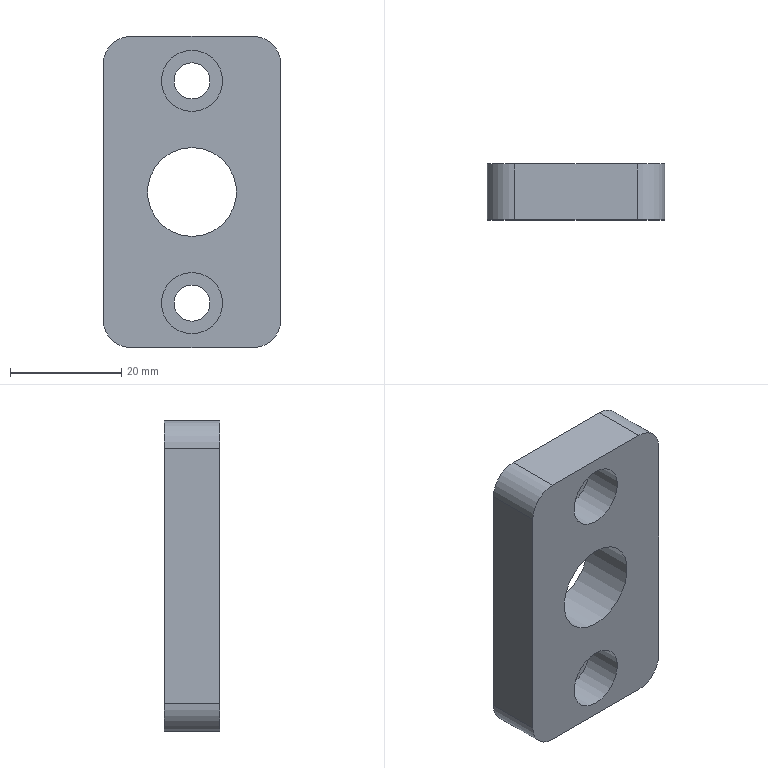Part | STEP file | B-PLATE-INSERT_id78_x_t | 1 solid | 17 faces | box 32 x 10 x 56 mm | volume 14165 mm3 | cylinder 9 | plane 8 | commonest cylinder face diameters 10 x4 6.5 x2 11 x2 16 x1
STEP:
#1=CARTESIAN_POINT('',(-115.,-113.5,-20.5));
#2=VERTEX_POINT('',#1);
#3=CARTESIAN_POINT('',(-115.,-113.5,-15.));
#4=DIRECTION('',(0.,-1.,0.));
#5=DIRECTION('',(0.,0.,-1.));
#6=AXIS2_PLACEMENT_3D('',#3,#4,#5);
#7=CIRCLE('',#6,5.5);
#8=EDGE_CURVE('',#2,#2,#7,.T.);
#9=ORIENTED_EDGE('',*,*,#8,.F.);
#10=EDGE_LOOP('',(#9));
#11=FACE_BOUND('',#10,.T.);
#12=CARTESIAN_POINT('',(-115.,-120.5,-20.5));
#13=VERTEX_POINT('',#12);
#14=CARTESIAN_POINT('',(-115.,-120.5,-15.));
#15=DIRECTION('',(0.,1.,0.));
#16=DIRECTION('',(0.,0.,-1.));
#17=AXIS2_PLACEMENT_3D('',#14,#15,#16);
#18=CIRCLE('',#17,5.5);
#19=EDGE_CURVE('',#13,#13,#18,.T.);
#20=ORIENTED_EDGE('',*,*,#19,.F.);
#21=EDGE_LOOP('',(#20));
#22=FACE_BOUND('',#21,.T.);
#23=CARTESIAN_POINT('',(-115.,-120.5,-15.));
#24=DIRECTION('',(0.,-1.,0.));
#25=DIRECTION('',(0.,0.,-1.));
#26=AXIS2_PLACEMENT_3D('',#23,#24,#25);
#27=CYLINDRICAL_SURFACE('',#26,5.5);
#28=ADVANCED_FACE('',(#11,#22),#27,.F.);
#29=CARTESIAN_POINT('',(-115.,-113.5,-60.5));
#30=VERTEX_POINT('',#29);
#31=CARTESIAN_POINT('',(-115.,-113.5,-55.));
#32=DIRECTION('',(0.,-1.,0.));
#33=DIRECTION('',(0.,0.,-1.));
#34=AXIS2_PLACEMENT_3D('',#31,#32,#33);
#35=CIRCLE('',#34,5.5);
#36=EDGE_CURVE('',#30,#30,#35,.T.);
#37=ORIENTED_EDGE('',*,*,#36,.F.);
#38=EDGE_LOOP('',(#37));
#39=FACE_BOUND('',#38,.T.);
#40=CARTESIAN_POINT('',(-115.,-120.5,-60.5));
#41=VERTEX_POINT('',#40);
#42=CARTESIAN_POINT('',(-115.,-120.5,-55.));
#43=DIRECTION('',(0.,1.,0.));
#44=DIRECTION('',(0.,0.,-1.));
#45=AXIS2_PLACEMENT_3D('',#42,#43,#44);
#46=CIRCLE('',#45,5.5);
#47=EDGE_CURVE('',#41,#41,#46,.T.);
#48=ORIENTED_EDGE('',*,*,#47,.F.);
#49=EDGE_LOOP('',(#48));
#50=FACE_BOUND('',#49,.T.);
#51=CARTESIAN_POINT('',(-115.,-120.5,-55.));
#52=DIRECTION('',(0.,-1.,0.));
#53=DIRECTION('',(0.,0.,-1.));
#54=AXIS2_PLACEMENT_3D('',#51,#52,#53);
#55=CYLINDRICAL_SURFACE('',#54,5.5);
#56=ADVANCED_FACE('',(#39,#50),#55,.F.);
#57=CARTESIAN_POINT('',(-115.,-120.5,-43.));
#58=VERTEX_POINT('',#57);
#59=CARTESIAN_POINT('',(-115.,-120.5,-35.));
#60=DIRECTION('',(0.,-1.,0.));
#61=DIRECTION('',(0.,0.,-1.));
#62=AXIS2_PLACEMENT_3D('',#59,#60,#61);
#63=CIRCLE('',#62,8.);
#64=EDGE_CURVE('',#58,#58,#63,.T.);
#65=ORIENTED_EDGE('',*,*,#64,.F.);
#66=EDGE_LOOP('',(#65));
#67=FACE_BOUND('',#66,.T.);
#68=ORIENTED_EDGE('',*,*,#19,.T.);
#69=EDGE_LOOP('',(#68));
#70=FACE_BOUND('',#69,.T.);
#71=ORIENTED_EDGE('',*,*,#47,.T.);
#72=EDGE_LOOP('',(#71));
#73=FACE_BOUND('',#72,.T.);
#74=CARTESIAN_POINT('',(-131.,-120.5,-58.));
#75=VERTEX_POINT('',#74);
#76=CARTESIAN_POINT('',(-131.,-120.5,-12.));
#77=VERTEX_POINT('',#76);
#78=CARTESIAN_POINT('',(-131.,-120.5,-12.));
#79=DIRECTION('',(0.,0.,1.));
#80=VECTOR('',#79,1.);
#81=LINE('',#78,#80);
#82=EDGE_CURVE('',#75,#77,#81,.T.);
#83=ORIENTED_EDGE('',*,*,#82,.F.);
#84=CARTESIAN_POINT('',(-126.,-120.5,-63.));
#85=VERTEX_POINT('',#84);
#86=CARTESIAN_POINT('',(-126.,-120.5,-58.));
#87=DIRECTION('',(0.,1.,0.));
#88=DIRECTION('',(0.,0.,-1.));
#89=AXIS2_PLACEMENT_3D('',#86,#87,#88);
#90=CIRCLE('',#89,5.);
#91=EDGE_CURVE('',#85,#75,#90,.T.);
#92=ORIENTED_EDGE('',*,*,#91,.F.);
#93=CARTESIAN_POINT('',(-104.,-120.5,-63.));
#94=VERTEX_POINT('',#93);
#95=CARTESIAN_POINT('',(-126.,-120.5,-63.));
#96=DIRECTION('',(-1.,0.,0.));
#97=VECTOR('',#96,1.);
#98=LINE('',#95,#97);
#99=EDGE_CURVE('',#94,#85,#98,.T.);
#100=ORIENTED_EDGE('',*,*,#99,.F.);
#101=CARTESIAN_POINT('',(-99.,-120.5,-58.));
#102=VERTEX_POINT('',#101);
#103=CARTESIAN_POINT('',(-104.,-120.5,-58.));
#104=DIRECTION('',(0.,1.,0.));
#105=DIRECTION('',(0.,0.,-1.));
#106=AXIS2_PLACEMENT_3D('',#103,#104,#105);
#107=CIRCLE('',#106,5.);
#108=EDGE_CURVE('',#102,#94,#107,.T.);
#109=ORIENTED_EDGE('',*,*,#108,.F.);
#110=CARTESIAN_POINT('',(-99.,-120.5,-12.));
#111=VERTEX_POINT('',#110);
#112=CARTESIAN_POINT('',(-99.,-120.5,-58.));
#113=DIRECTION('',(0.,0.,-1.));
#114=VECTOR('',#113,1.);
#115=LINE('',#112,#114);
#116=EDGE_CURVE('',#111,#102,#115,.T.);
#117=ORIENTED_EDGE('',*,*,#116,.F.);
#118=CARTESIAN_POINT('',(-104.,-120.5,-7.));
#119=VERTEX_POINT('',#118);
#120=CARTESIAN_POINT('',(-104.,-120.5,-12.));
#121=DIRECTION('',(0.,1.,0.));
#122=DIRECTION('',(0.,0.,-1.));
#123=AXIS2_PLACEMENT_3D('',#120,#121,#122);
#124=CIRCLE('',#123,5.);
#125=EDGE_CURVE('',#119,#111,#124,.T.);
#126=ORIENTED_EDGE('',*,*,#125,.F.);
#127=CARTESIAN_POINT('',(-126.,-120.5,-7.));
#128=VERTEX_POINT('',#127);
#129=CARTESIAN_POINT('',(-104.,-120.5,-7.));
#130=DIRECTION('',(1.,0.,0.));
#131=VECTOR('',#130,1.);
#132=LINE('',#129,#131);
#133=EDGE_CURVE('',#128,#119,#132,.T.);
#134=ORIENTED_EDGE('',*,*,#133,.F.);
#135=CARTESIAN_POINT('',(-126.,-120.5,-12.));
#136=DIRECTION('',(0.,1.,0.));
#137=DIRECTION('',(0.,0.,-1.));
#138=AXIS2_PLACEMENT_3D('',#135,#136,#137);
#139=CIRCLE('',#138,5.);
#140=EDGE_CURVE('',#77,#128,#139,.T.);
#141=ORIENTED_EDGE('',*,*,#140,.F.);
#142=EDGE_LOOP('',(#83,#92,#100,#109,#117,#126,#134,#141));
#143=FACE_BOUND('',#142,.T.);
#144=CARTESIAN_POINT('',(-80.,-120.5,-43.));
#145=DIRECTION('',(0.,-1.,0.));
#146=DIRECTION('',(0.,0.,-1.));
#147=AXIS2_PLACEMENT_3D('',#144,#145,#146);
#148=PLANE('',#147);
#149=ADVANCED_FACE('',(#67,#70,#73,#143),#148,.T.);
#150=CARTESIAN_POINT('',(-115.,-113.5,-18.25));
#151=VERTEX_POINT('',#150);
#152=CARTESIAN_POINT('',(-115.,-113.5,-15.));
#153=DIRECTION('',(0.,1.,0.));
#154=DIRECTION('',(0.,0.,-1.));
#155=AXIS2_PLACEMENT_3D('',#152,#153,#154);
#156=CIRCLE('',#155,3.25);
#157=EDGE_CURVE('',#151,#151,#156,.T.);
#158=ORIENTED_EDGE('',*,*,#157,.T.);
#159=EDGE_LOOP('',(#158));
#160=FACE_BOUND('',#159,.T.);
#161=ORIENTED_EDGE('',*,*,#8,.T.);
#162=EDGE_LOOP('',(#161));
#163=FACE_BOUND('',#162,.T.);
#164=CARTESIAN_POINT('',(-200.,-113.5,-275.));
#165=DIRECTION('',(0.,-1.,0.));
#166=DIRECTION('',(0.,0.,-1.));
#167=AXIS2_PLACEMENT_3D('',#164,#165,#166);
#168=PLANE('',#167);
#169=ADVANCED_FACE('',(#160,#163),#168,.T.);
#170=CARTESIAN_POINT('',(-115.,-113.5,-58.25));
#171=VERTEX_POINT('',#170);
#172=CARTESIAN_POINT('',(-115.,-113.5,-55.));
#173=DIRECTION('',(0.,1.,0.));
#174=DIRECTION('',(0.,0.,-1.));
#175=AXIS2_PLACEMENT_3D('',#172,#173,#174);
#176=CIRCLE('',#175,3.25);
#177=EDGE_CURVE('',#171,#171,#176,.T.);
#178=ORIENTED_EDGE('',*,*,#177,.T.);
#179=EDGE_LOOP('',(#178));
#180=FACE_BOUND('',#179,.T.);
#181=ORIENTED_EDGE('',*,*,#36,.T.);
#182=EDGE_LOOP('',(#181));
#183=FACE_BOUND('',#182,.T.);
#184=CARTESIAN_POINT('',(-200.,-113.5,-275.));
#185=DIRECTION('',(0.,-1.,0.));
#186=DIRECTION('',(0.,0.,-1.));
#187=AXIS2_PLACEMENT_3D('',#184,#185,#186);
#188=PLANE('',#187);
#189=ADVANCED_FACE('',(#180,#183),#188,.T.);
#190=CARTESIAN_POINT('',(-131.,-110.5,-58.));
#191=VERTEX_POINT('',#190);
#192=CARTESIAN_POINT('',(-131.,-110.5,-58.));
#193=DIRECTION('',(0.,-1.,0.));
#194=VECTOR('',#193,1.);
#195=LINE('',#192,#194);
#196=EDGE_CURVE('',#191,#75,#195,.T.);
#197=ORIENTED_EDGE('',*,*,#196,.F.);
#198=CARTESIAN_POINT('',(-126.,-110.5,-63.));
#199=VERTEX_POINT('',#198);
#200=CARTESIAN_POINT('',(-126.,-110.5,-58.));
#201=DIRECTION('',(0.,-1.,0.));
#202=DIRECTION('',(0.,0.,-1.));
#203=AXIS2_PLACEMENT_3D('',#200,#201,#202);
#204=CIRCLE('',#203,5.);
#205=EDGE_CURVE('',#191,#199,#204,.T.);
#206=ORIENTED_EDGE('',*,*,#205,.T.);
#207=CARTESIAN_POINT('',(-126.,-110.5,-63.));
#208=DIRECTION('',(0.,1.,0.));
#209=VECTOR('',#208,1.);
#210=LINE('',#207,#209);
#211=EDGE_CURVE('',#85,#199,#210,.T.);
#212=ORIENTED_EDGE('',*,*,#211,.F.);
#213=ORIENTED_EDGE('',*,*,#91,.T.);
#214=EDGE_LOOP('',(#197,#206,#212,#213));
#215=FACE_OUTER_BOUND('',#214,.T.);
#216=CARTESIAN_POINT('',(-126.,-110.5,-58.));
#217=DIRECTION('',(0.,-1.,0.));
#218=DIRECTION('',(0.,0.,-1.));
#219=AXIS2_PLACEMENT_3D('',#216,#217,#218);
#220=CYLINDRICAL_SURFACE('',#219,5.);
#221=ADVANCED_FACE('',(#215),#220,.T.);
#222=ORIENTED_EDGE('',*,*,#211,.T.);
#223=CARTESIAN_POINT('',(-104.,-110.5,-63.));
#224=VERTEX_POINT('',#223);
#225=CARTESIAN_POINT('',(-200.,-110.5,-63.));
#226=DIRECTION('',(1.,0.,0.));
#227=VECTOR('',#226,1.);
#228=LINE('',#225,#227);
#229=EDGE_CURVE('',#199,#224,#228,.T.);
#230=ORIENTED_EDGE('',*,*,#229,.T.);
#231=CARTESIAN_POINT('',(-104.,-110.5,-63.));
#232=DIRECTION('',(0.,1.,0.));
#233=VECTOR('',#232,1.);
#234=LINE('',#231,#233);
#235=EDGE_CURVE('',#94,#224,#234,.T.);
#236=ORIENTED_EDGE('',*,*,#235,.F.);
#237=ORIENTED_EDGE('',*,*,#99,.T.);
#238=EDGE_LOOP('',(#222,#230,#236,#237));
#239=FACE_OUTER_BOUND('',#238,.T.);
#240=CARTESIAN_POINT('',(-126.,-110.5,-63.));
#241=DIRECTION('',(0.,0.,-1.));
#242=DIRECTION('',(-1.,0.,0.));
#243=AXIS2_PLACEMENT_3D('',#240,#241,#242);
#244=PLANE('',#243);
#245=ADVANCED_FACE('',(#239),#244,.T.);
#246=ORIENTED_EDGE('',*,*,#235,.T.);
#247=CARTESIAN_POINT('',(-99.,-110.5,-58.));
#248=VERTEX_POINT('',#247);
#249=CARTESIAN_POINT('',(-104.,-110.5,-58.));
#250=DIRECTION('',(0.,-1.,0.));
#251=DIRECTION('',(0.,0.,-1.));
#252=AXIS2_PLACEMENT_3D('',#249,#250,#251);
#253=CIRCLE('',#252,5.);
#254=EDGE_CURVE('',#224,#248,#253,.T.);
#255=ORIENTED_EDGE('',*,*,#254,.T.);
#256=CARTESIAN_POINT('',(-99.,-110.5,-58.));
#257=DIRECTION('',(0.,1.,0.));
#258=VECTOR('',#257,1.);
#259=LINE('',#256,#258);
#260=EDGE_CURVE('',#102,#248,#259,.T.);
#261=ORIENTED_EDGE('',*,*,#260,.F.);
#262=ORIENTED_EDGE('',*,*,#108,.T.);
#263=EDGE_LOOP('',(#246,#255,#261,#262));
#264=FACE_OUTER_BOUND('',#263,.T.);
#265=CARTESIAN_POINT('',(-104.,-110.5,-58.));
#266=DIRECTION('',(0.,-1.,0.));
#267=DIRECTION('',(0.,0.,-1.));
#268=AXIS2_PLACEMENT_3D('',#265,#266,#267);
#269=CYLINDRICAL_SURFACE('',#268,5.);
#270=ADVANCED_FACE('',(#264),#269,.T.);
#271=ORIENTED_EDGE('',*,*,#260,.T.);
#272=CARTESIAN_POINT('',(-99.,-110.5,-12.));
#273=VERTEX_POINT('',#272);
#274=CARTESIAN_POINT('',(-99.,-110.5,-275.));
#275=DIRECTION('',(0.,0.,1.));
#276=VECTOR('',#275,1.);
#277=LINE('',#274,#276);
#278=EDGE_CURVE('',#248,#273,#277,.T.);
#279=ORIENTED_EDGE('',*,*,#278,.T.);
#280=CARTESIAN_POINT('',(-99.,-110.5,-12.));
#281=DIRECTION('',(0.,1.,0.));
#282=VECTOR('',#281,1.);
#283=LINE('',#280,#282);
#284=EDGE_CURVE('',#111,#273,#283,.T.);
#285=ORIENTED_EDGE('',*,*,#284,.F.);
#286=ORIENTED_EDGE('',*,*,#116,.T.);
#287=EDGE_LOOP('',(#271,#279,#285,#286));
#288=FACE_OUTER_BOUND('',#287,.T.);
#289=CARTESIAN_POINT('',(-99.,-110.5,-58.));
#290=DIRECTION('',(1.,0.,0.));
#291=DIRECTION('',(0.,0.,-1.));
#292=AXIS2_PLACEMENT_3D('',#289,#290,#291);
#293=PLANE('',#292);
#294=ADVANCED_FACE('',(#288),#293,.T.);
#295=ORIENTED_EDGE('',*,*,#284,.T.);
#296=CARTESIAN_POINT('',(-104.,-110.5,-7.));
#297=VERTEX_POINT('',#296);
#298=CARTESIAN_POINT('',(-104.,-110.5,-12.));
#299=DIRECTION('',(0.,-1.,0.));
#300=DIRECTION('',(0.,0.,-1.));
#301=AXIS2_PLACEMENT_3D('',#298,#299,#300);
#302=CIRCLE('',#301,5.);
#303=EDGE_CURVE('',#273,#297,#302,.T.);
#304=ORIENTED_EDGE('',*,*,#303,.T.);
#305=CARTESIAN_POINT('',(-104.,-110.5,-7.));
#306=DIRECTION('',(0.,1.,0.));
#307=VECTOR('',#306,1.);
#308=LINE('',#305,#307);
#309=EDGE_CURVE('',#119,#297,#308,.T.);
#310=ORIENTED_EDGE('',*,*,#309,.F.);
#311=ORIENTED_EDGE('',*,*,#125,.T.);
#312=EDGE_LOOP('',(#295,#304,#310,#311));
#313=FACE_OUTER_BOUND('',#312,.T.);
#314=CARTESIAN_POINT('',(-104.,-110.5,-12.));
#315=DIRECTION('',(0.,-1.,0.));
#316=DIRECTION('',(0.,0.,-1.));
#317=AXIS2_PLACEMENT_3D('',#314,#315,#316);
#318=CYLINDRICAL_SURFACE('',#317,5.);
#319=ADVANCED_FACE('',(#313),#318,.T.);
#320=ORIENTED_EDGE('',*,*,#309,.T.);
#321=CARTESIAN_POINT('',(-126.,-110.5,-7.));
#322=VERTEX_POINT('',#321);
#323=CARTESIAN_POINT('',(-200.,-110.5,-7.));
#324=DIRECTION('',(-1.,0.,0.));
#325=VECTOR('',#324,1.);
#326=LINE('',#323,#325);
#327=EDGE_CURVE('',#297,#322,#326,.T.);
#328=ORIENTED_EDGE('',*,*,#327,.T.);
#329=CARTESIAN_POINT('',(-126.,-110.5,-7.));
#330=DIRECTION('',(0.,1.,0.));
#331=VECTOR('',#330,1.);
#332=LINE('',#329,#331);
#333=EDGE_CURVE('',#128,#322,#332,.T.);
#334=ORIENTED_EDGE('',*,*,#333,.F.);
#335=ORIENTED_EDGE('',*,*,#133,.T.);
#336=EDGE_LOOP('',(#320,#328,#334,#335));
#337=FACE_OUTER_BOUND('',#336,.T.);
#338=CARTESIAN_POINT('',(-104.,-110.5,-7.));
#339=DIRECTION('',(0.,0.,1.));
#340=DIRECTION('',(1.,0.,0.));
#341=AXIS2_PLACEMENT_3D('',#338,#339,#340);
#342=PLANE('',#341);
#343=ADVANCED_FACE('',(#337),#342,.T.);
#344=ORIENTED_EDGE('',*,*,#333,.T.);
#345=CARTESIAN_POINT('',(-131.,-110.5,-12.));
#346=VERTEX_POINT('',#345);
#347=CARTESIAN_POINT('',(-126.,-110.5,-12.));
#348=DIRECTION('',(0.,-1.,0.));
#349=DIRECTION('',(0.,0.,-1.));
#350=AXIS2_PLACEMENT_3D('',#347,#348,#349);
#351=CIRCLE('',#350,5.);
#352=EDGE_CURVE('',#322,#346,#351,.T.);
#353=ORIENTED_EDGE('',*,*,#352,.T.);
#354=CARTESIAN_POINT('',(-131.,-110.5,-12.));
#355=DIRECTION('',(0.,1.,0.));
#356=VECTOR('',#355,1.);
#357=LINE('',#354,#356);
#358=EDGE_CURVE('',#77,#346,#357,.T.);
#359=ORIENTED_EDGE('',*,*,#358,.F.);
#360=ORIENTED_EDGE('',*,*,#140,.T.);
#361=EDGE_LOOP('',(#344,#353,#359,#360));
#362=FACE_OUTER_BOUND('',#361,.T.);
#363=CARTESIAN_POINT('',(-126.,-110.5,-12.));
#364=DIRECTION('',(0.,-1.,0.));
#365=DIRECTION('',(0.,0.,-1.));
#366=AXIS2_PLACEMENT_3D('',#363,#364,#365);
#367=CYLINDRICAL_SURFACE('',#366,5.);
#368=ADVANCED_FACE('',(#362),#367,.T.);
#369=ORIENTED_EDGE('',*,*,#358,.T.);
#370=CARTESIAN_POINT('',(-131.,-110.5,-275.));
#371=DIRECTION('',(0.,0.,-1.));
#372=VECTOR('',#371,1.);
#373=LINE('',#370,#372);
#374=EDGE_CURVE('',#346,#191,#373,.T.);
#375=ORIENTED_EDGE('',*,*,#374,.T.);
#376=ORIENTED_EDGE('',*,*,#196,.T.);
#377=ORIENTED_EDGE('',*,*,#82,.T.);
#378=EDGE_LOOP('',(#369,#375,#376,#377));
#379=FACE_OUTER_BOUND('',#378,.T.);
#380=CARTESIAN_POINT('',(-131.,-110.5,-12.));
#381=DIRECTION('',(-1.,0.,0.));
#382=DIRECTION('',(0.,0.,1.));
#383=AXIS2_PLACEMENT_3D('',#380,#381,#382);
#384=PLANE('',#383);
#385=ADVANCED_FACE('',(#379),#384,.T.);
#386=CARTESIAN_POINT('',(-115.,-110.5,-18.25));
#387=VERTEX_POINT('',#386);
#388=CARTESIAN_POINT('',(-115.,-110.5,-15.));
#389=DIRECTION('',(0.,1.,0.));
#390=DIRECTION('',(0.,0.,-1.));
#391=AXIS2_PLACEMENT_3D('',#388,#389,#390);
#392=CIRCLE('',#391,3.25);
#393=EDGE_CURVE('',#387,#387,#392,.T.);
#394=ORIENTED_EDGE('',*,*,#393,.T.);
#395=EDGE_LOOP('',(#394));
#396=FACE_BOUND('',#395,.T.);
#397=ORIENTED_EDGE('',*,*,#157,.F.);
#398=EDGE_LOOP('',(#397));
#399=FACE_BOUND('',#398,.T.);
#400=CARTESIAN_POINT('',(-115.,-120.5,-15.));
#401=DIRECTION('',(0.,-1.,0.));
#402=DIRECTION('',(0.,0.,-1.));
#403=AXIS2_PLACEMENT_3D('',#400,#401,#402);
#404=CYLINDRICAL_SURFACE('',#403,3.25);
#405=ADVANCED_FACE('',(#396,#399),#404,.F.);
#406=CARTESIAN_POINT('',(-115.,-110.5,-58.25));
#407=VERTEX_POINT('',#406);
#408=CARTESIAN_POINT('',(-115.,-110.5,-55.));
#409=DIRECTION('',(0.,1.,0.));
#410=DIRECTION('',(0.,0.,-1.));
#411=AXIS2_PLACEMENT_3D('',#408,#409,#410);
#412=CIRCLE('',#411,3.25);
#413=EDGE_CURVE('',#407,#407,#412,.T.);
#414=ORIENTED_EDGE('',*,*,#413,.T.);
#415=EDGE_LOOP('',(#414));
#416=FACE_BOUND('',#415,.T.);
#417=ORIENTED_EDGE('',*,*,#177,.F.);
#418=EDGE_LOOP('',(#417));
#419=FACE_BOUND('',#418,.T.);
#420=CARTESIAN_POINT('',(-115.,-120.5,-55.));
#421=DIRECTION('',(0.,-1.,0.));
#422=DIRECTION('',(0.,0.,-1.));
#423=AXIS2_PLACEMENT_3D('',#420,#421,#422);
#424=CYLINDRICAL_SURFACE('',#423,3.25);
#425=ADVANCED_FACE('',(#416,#419),#424,.F.);
#426=CARTESIAN_POINT('',(-115.,-110.5,-43.));
#427=VERTEX_POINT('',#426);
#428=CARTESIAN_POINT('',(-115.,-110.5,-35.));
#429=DIRECTION('',(0.,-1.,0.));
#430=DIRECTION('',(0.,0.,-1.));
#431=AXIS2_PLACEMENT_3D('',#428,#429,#430);
#432=CIRCLE('',#431,8.);
#433=EDGE_CURVE('',#427,#427,#432,.T.);
#434=ORIENTED_EDGE('',*,*,#433,.T.);
#435=EDGE_LOOP('',(#434));
#436=FACE_BOUND('',#435,.T.);
#437=ORIENTED_EDGE('',*,*,#413,.F.);
#438=EDGE_LOOP('',(#437));
#439=FACE_BOUND('',#438,.T.);
#440=ORIENTED_EDGE('',*,*,#393,.F.);
#441=EDGE_LOOP('',(#440));
#442=FACE_BOUND('',#441,.T.);
#443=ORIENTED_EDGE('',*,*,#352,.F.);
#444=ORIENTED_EDGE('',*,*,#327,.F.);
#445=ORIENTED_EDGE('',*,*,#303,.F.);
#446=ORIENTED_EDGE('',*,*,#278,.F.);
#447=ORIENTED_EDGE('',*,*,#254,.F.);
#448=ORIENTED_EDGE('',*,*,#229,.F.);
#449=ORIENTED_EDGE('',*,*,#205,.F.);
#450=ORIENTED_EDGE('',*,*,#374,.F.);
#451=EDGE_LOOP('',(#443,#444,#445,#446,#447,#448,#449,#450));
#452=FACE_BOUND('',#451,.T.);
#453=CARTESIAN_POINT('',(-200.,-110.5,-275.));
#454=DIRECTION('',(0.,-1.,0.));
#455=DIRECTION('',(0.,0.,-1.));
#456=AXIS2_PLACEMENT_3D('',#453,#454,#455);
#457=PLANE('',#456);
#458=ADVANCED_FACE('',(#436,#439,#442,#452),#457,.F.);
#459=ORIENTED_EDGE('',*,*,#64,.T.);
#460=EDGE_LOOP('',(#459));
#461=FACE_BOUND('',#460,.T.);
#462=ORIENTED_EDGE('',*,*,#433,.F.);
#463=EDGE_LOOP('',(#462));
#464=FACE_BOUND('',#463,.T.);
#465=CARTESIAN_POINT('',(-115.,-231.55,-35.));
#466=DIRECTION('',(0.,1.,0.));
#467=DIRECTION('',(0.,0.,1.));
#468=AXIS2_PLACEMENT_3D('',#465,#466,#467);
#469=CYLINDRICAL_SURFACE('',#468,8.);
#470=ADVANCED_FACE('',(#461,#464),#469,.F.);
#471=CLOSED_SHELL('',(#28,#56,#149,#169,#189,#221,#245,#270,#294,#319,#343,#368,#385,#405,#425,#458,#470));
#472=MANIFOLD_SOLID_BREP('',#471);
#473=(LENGTH_UNIT()NAMED_UNIT(*)SI_UNIT(.MILLI.,.METRE.));
#474=UNCERTAINTY_MEASURE_WITH_UNIT(LENGTH_MEASURE(0.00002),#473,'','');
#475=(NAMED_UNIT(*)PLANE_ANGLE_UNIT()SI_UNIT($,.RADIAN.));
#476=PLANE_ANGLE_MEASURE_WITH_UNIT(PLANE_ANGLE_MEASURE(0.01745),#475);
#477=DIMENSIONAL_EXPONENTS(0.,0.,0.,0.,0.,0.,0.);
#478=(CONVERSION_BASED_UNIT('DEGREE',#476)NAMED_UNIT(#477)PLANE_ANGLE_UNIT());
#479=(NAMED_UNIT(*)SI_UNIT($,.STERADIAN.)SOLID_ANGLE_UNIT());
#480=(GEOMETRIC_REPRESENTATION_CONTEXT(3)GLOBAL_UNCERTAINTY_ASSIGNED_CONTEXT((#474))GLOBAL_UNIT_ASSIGNED_CONTEXT((#473,#478,#479))REPRESENTATION_CONTEXT('',''));
#481=ADVANCED_BREP_SHAPE_REPRESENTATION('',(#472),#480);